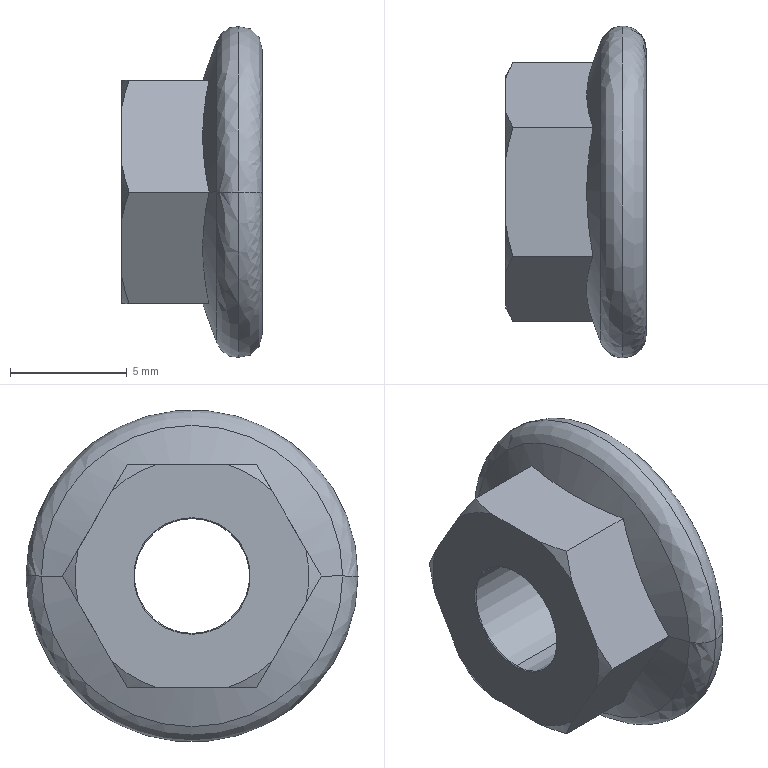Part | SolidWorks | features BaseBody 1 | 1 solid | 26 faces | box 6 x 14.2 x 14.2 mm | volume 511.274 mm3 | cone 12 | plane 8 | spline 4 | cylinder 2 | commonest cylinder face diameters 4.918 x2
STEP:
#1=CARTESIAN_POINT('',(-1.,7.1,0.));
#2=VERTEX_POINT('',#1);
#3=CARTESIAN_POINT('',(-1.,-7.1,0.));
#4=VERTEX_POINT('',#3);
#5=CARTESIAN_POINT('',(-1.,0.,0.));
#6=DIRECTION('',(-1.,0.,0.));
#7=DIRECTION('',(0.,-1.,0.));
#8=AXIS2_PLACEMENT_3D('',#5,#6,#7);
#9=CIRCLE('',#8,7.1);
#10=EDGE_CURVE('',#2,#4,#9,.T.);
#11=ORIENTED_EDGE('',*,*,#10,.F.);
#12=CARTESIAN_POINT('',(0.,6.1,0.));
#13=VERTEX_POINT('',#12);
#14=CARTESIAN_POINT('',(-1.,6.1,0.));
#15=DIRECTION('',(0.,0.,-1.));
#16=DIRECTION('',(0.,1.,0.));
#17=AXIS2_PLACEMENT_3D('',#14,#15,#16);
#18=CIRCLE('',#17,1.);
#19=EDGE_CURVE('',#2,#13,#18,.T.);
#20=ORIENTED_EDGE('',*,*,#19,.T.);
#21=CARTESIAN_POINT('',(0.,-6.1,0.));
#22=VERTEX_POINT('',#21);
#23=CARTESIAN_POINT('',(0.,6.1,0.));
#24=CARTESIAN_POINT('',(0.,6.1,-12.2));
#25=CARTESIAN_POINT('',(0.,-6.1,-12.2));
#26=CARTESIAN_POINT('',(0.,-6.1,0.));
#27=(BOUNDED_CURVE()B_SPLINE_CURVE(3,(#23,#24,#25,#26),.UNSPECIFIED.,.F.,.F.)B_SPLINE_CURVE_WITH_KNOTS((4,4),(0.,1.),.UNSPECIFIED.)CURVE()GEOMETRIC_REPRESENTATION_ITEM()RATIONAL_B_SPLINE_CURVE((1.,0.3333,0.3333,1.))REPRESENTATION_ITEM(''));
#28=EDGE_CURVE('',#13,#22,#27,.T.);
#29=ORIENTED_EDGE('',*,*,#28,.T.);
#30=CARTESIAN_POINT('',(-1.,-6.1,0.));
#31=DIRECTION('',(0.,0.,1.));
#32=DIRECTION('',(0.,-1.,0.));
#33=AXIS2_PLACEMENT_3D('',#30,#31,#32);
#34=CIRCLE('',#33,1.);
#35=EDGE_CURVE('',#4,#22,#34,.T.);
#36=ORIENTED_EDGE('',*,*,#35,.F.);
#37=EDGE_LOOP('',(#11,#20,#29,#36));
#38=FACE_OUTER_BOUND('',#37,.T.);
#39=CARTESIAN_POINT('',(-1.,7.1,0.));
#40=CARTESIAN_POINT('',(-1.,7.1,-14.2));
#41=CARTESIAN_POINT('',(-1.,-7.1,-14.2));
#42=CARTESIAN_POINT('',(-1.,-7.1,0.));
#43=CARTESIAN_POINT('',(-0.4142,7.1,0.));
#44=CARTESIAN_POINT('',(-0.4142,7.1,-14.2));
#45=CARTESIAN_POINT('',(-0.4142,-7.1,-14.2));
#46=CARTESIAN_POINT('',(-0.4142,-7.1,0.));
#47=CARTESIAN_POINT('',(0.,6.686,0.));
#48=CARTESIAN_POINT('',(0.,6.686,-13.372));
#49=CARTESIAN_POINT('',(0.,-6.686,-13.372));
#50=CARTESIAN_POINT('',(0.,-6.686,0.));
#51=CARTESIAN_POINT('',(0.,6.1,0.));
#52=CARTESIAN_POINT('',(0.,6.1,-12.2));
#53=CARTESIAN_POINT('',(0.,-6.1,-12.2));
#54=CARTESIAN_POINT('',(0.,-6.1,0.));
#55=(BOUNDED_SURFACE()B_SPLINE_SURFACE(3,3,((#39,#40,#41,#42),(#43,#44,#45,#46),(#47,#48,#49,#50),(#51,#52,#53,#54)),.UNSPECIFIED.,.F.,.F.,.T.)B_SPLINE_SURFACE_WITH_KNOTS((4,4),(4,4),(0.,1.),(0.,1.),.UNSPECIFIED.)GEOMETRIC_REPRESENTATION_ITEM()RATIONAL_B_SPLINE_SURFACE(((1.,0.3333,0.3333,1.),(0.8047,0.2682,0.2682,0.8047),(0.8047,0.2682,0.2682,0.8047),(1.,0.3333,0.3333,1.)))REPRESENTATION_ITEM('')SURFACE());
#56=ADVANCED_FACE('',(#38),#55,.T.);
#57=CARTESIAN_POINT('',(-1.94,-6.442,0.));
#58=VERTEX_POINT('',#57);
#59=CARTESIAN_POINT('',(-1.94,6.442,0.));
#60=VERTEX_POINT('',#59);
#61=CARTESIAN_POINT('',(-1.94,0.,0.));
#62=DIRECTION('',(1.,0.,0.));
#63=DIRECTION('',(0.,-1.,0.));
#64=AXIS2_PLACEMENT_3D('',#61,#62,#63);
#65=CIRCLE('',#64,6.442);
#66=EDGE_CURVE('',#58,#60,#65,.T.);
#67=ORIENTED_EDGE('',*,*,#66,.T.);
#68=CARTESIAN_POINT('',(-1.,6.1,0.));
#69=DIRECTION('',(0.,0.,-1.));
#70=DIRECTION('',(0.,1.,0.));
#71=AXIS2_PLACEMENT_3D('',#68,#69,#70);
#72=CIRCLE('',#71,1.);
#73=EDGE_CURVE('',#60,#2,#72,.T.);
#74=ORIENTED_EDGE('',*,*,#73,.T.);
#75=ORIENTED_EDGE('',*,*,#10,.T.);
#76=CARTESIAN_POINT('',(-1.,-6.1,0.));
#77=DIRECTION('',(0.,0.,1.));
#78=DIRECTION('',(0.,-1.,0.));
#79=AXIS2_PLACEMENT_3D('',#76,#77,#78);
#80=CIRCLE('',#79,1.);
#81=EDGE_CURVE('',#58,#4,#80,.T.);
#82=ORIENTED_EDGE('',*,*,#81,.F.);
#83=EDGE_LOOP('',(#67,#74,#75,#82));
#84=FACE_OUTER_BOUND('',#83,.T.);
#85=CARTESIAN_POINT('',(-1.94,6.442,0.));
#86=CARTESIAN_POINT('',(-1.94,6.442,-12.884));
#87=CARTESIAN_POINT('',(-1.94,-6.442,-12.884));
#88=CARTESIAN_POINT('',(-1.94,-6.442,0.));
#89=CARTESIAN_POINT('',(-1.791,6.851,0.));
#90=CARTESIAN_POINT('',(-1.791,6.851,-13.701));
#91=CARTESIAN_POINT('',(-1.791,-6.851,-13.701));
#92=CARTESIAN_POINT('',(-1.791,-6.851,0.));
#93=CARTESIAN_POINT('',(-1.435,7.1,0.));
#94=CARTESIAN_POINT('',(-1.435,7.1,-14.2));
#95=CARTESIAN_POINT('',(-1.435,-7.1,-14.2));
#96=CARTESIAN_POINT('',(-1.435,-7.1,0.));
#97=CARTESIAN_POINT('',(-1.,7.1,0.));
#98=CARTESIAN_POINT('',(-1.,7.1,-14.2));
#99=CARTESIAN_POINT('',(-1.,-7.1,-14.2));
#100=CARTESIAN_POINT('',(-1.,-7.1,0.));
#101=(BOUNDED_SURFACE()B_SPLINE_SURFACE(3,3,((#85,#86,#87,#88),(#89,#90,#91,#92),(#93,#94,#95,#96),(#97,#98,#99,#100)),.UNSPECIFIED.,.F.,.F.,.T.)B_SPLINE_SURFACE_WITH_KNOTS((4,4),(4,4),(0.,1.),(0.,1.),.UNSPECIFIED.)GEOMETRIC_REPRESENTATION_ITEM()RATIONAL_B_SPLINE_SURFACE(((1.,0.3333,0.3333,1.),(0.8794,0.2931,0.2931,0.8794),(0.8794,0.2931,0.2931,0.8794),(1.,0.3333,0.3333,1.)))REPRESENTATION_ITEM('')SURFACE());
#102=ADVANCED_FACE('',(#84),#101,.T.);
#103=ORIENTED_EDGE('',*,*,#73,.F.);
#104=CARTESIAN_POINT('',(-1.94,0.,0.));
#105=DIRECTION('',(1.,0.,0.));
#106=DIRECTION('',(0.,-1.,0.));
#107=AXIS2_PLACEMENT_3D('',#104,#105,#106);
#108=CIRCLE('',#107,6.442);
#109=EDGE_CURVE('',#60,#58,#108,.T.);
#110=ORIENTED_EDGE('',*,*,#109,.T.);
#111=ORIENTED_EDGE('',*,*,#81,.T.);
#112=CARTESIAN_POINT('',(-1.,0.,0.));
#113=DIRECTION('',(-1.,0.,0.));
#114=DIRECTION('',(0.,-1.,0.));
#115=AXIS2_PLACEMENT_3D('',#112,#113,#114);
#116=CIRCLE('',#115,7.1);
#117=EDGE_CURVE('',#4,#2,#116,.T.);
#118=ORIENTED_EDGE('',*,*,#117,.T.);
#119=EDGE_LOOP('',(#103,#110,#111,#118));
#120=FACE_OUTER_BOUND('',#119,.T.);
#121=CARTESIAN_POINT('',(-1.94,-6.442,0.));
#122=CARTESIAN_POINT('',(-1.94,-6.442,12.884));
#123=CARTESIAN_POINT('',(-1.94,6.442,12.884));
#124=CARTESIAN_POINT('',(-1.94,6.442,0.));
#125=CARTESIAN_POINT('',(-1.791,-6.851,0.));
#126=CARTESIAN_POINT('',(-1.791,-6.851,13.701));
#127=CARTESIAN_POINT('',(-1.791,6.851,13.701));
#128=CARTESIAN_POINT('',(-1.791,6.851,0.));
#129=CARTESIAN_POINT('',(-1.435,-7.1,0.));
#130=CARTESIAN_POINT('',(-1.435,-7.1,14.2));
#131=CARTESIAN_POINT('',(-1.435,7.1,14.2));
#132=CARTESIAN_POINT('',(-1.435,7.1,0.));
#133=CARTESIAN_POINT('',(-1.,-7.1,0.));
#134=CARTESIAN_POINT('',(-1.,-7.1,14.2));
#135=CARTESIAN_POINT('',(-1.,7.1,14.2));
#136=CARTESIAN_POINT('',(-1.,7.1,0.));
#137=(BOUNDED_SURFACE()B_SPLINE_SURFACE(3,3,((#121,#122,#123,#124),(#125,#126,#127,#128),(#129,#130,#131,#132),(#133,#134,#135,#136)),.UNSPECIFIED.,.F.,.F.,.T.)B_SPLINE_SURFACE_WITH_KNOTS((4,4),(4,4),(0.,1.),(0.,1.),.UNSPECIFIED.)GEOMETRIC_REPRESENTATION_ITEM()RATIONAL_B_SPLINE_SURFACE(((1.,0.3333,0.3333,1.),(0.8794,0.2931,0.2931,0.8794),(0.8794,0.2931,0.2931,0.8794),(1.,0.3333,0.3333,1.)))REPRESENTATION_ITEM('')SURFACE());
#138=ADVANCED_FACE('',(#120),#137,.T.);
#139=CARTESIAN_POINT('',(-0.03571,0.,2.459));
#140=VERTEX_POINT('',#139);
#141=CARTESIAN_POINT('',(-0.03571,0.,-2.459));
#142=VERTEX_POINT('',#141);
#143=CARTESIAN_POINT('',(-0.03571,0.,0.));
#144=DIRECTION('',(1.,0.,0.));
#145=DIRECTION('',(0.,0.,-1.));
#146=AXIS2_PLACEMENT_3D('',#143,#144,#145);
#147=CIRCLE('',#146,2.459);
#148=EDGE_CURVE('',#140,#142,#147,.T.);
#149=ORIENTED_EDGE('',*,*,#148,.F.);
#150=CARTESIAN_POINT('',(0.,0.,2.494));
#151=VERTEX_POINT('',#150);
#152=CARTESIAN_POINT('',(0.,0.,2.494));
#153=DIRECTION('',(0.7071,0.,0.7071));
#154=VECTOR('',#153,1000.);
#155=LINE('',#152,#154);
#156=EDGE_CURVE('',#140,#151,#155,.T.);
#157=ORIENTED_EDGE('',*,*,#156,.T.);
#158=CARTESIAN_POINT('',(0.,0.,-2.494));
#159=VERTEX_POINT('',#158);
#160=CARTESIAN_POINT('',(0.,0.,0.));
#161=DIRECTION('',(1.,0.,0.));
#162=DIRECTION('',(0.,0.,-1.));
#163=AXIS2_PLACEMENT_3D('',#160,#161,#162);
#164=CIRCLE('',#163,2.494);
#165=EDGE_CURVE('',#151,#159,#164,.T.);
#166=ORIENTED_EDGE('',*,*,#165,.T.);
#167=CARTESIAN_POINT('',(0.,0.,-2.494));
#168=DIRECTION('',(0.7071,0.,-0.7071));
#169=VECTOR('',#168,1000.);
#170=LINE('',#167,#169);
#171=EDGE_CURVE('',#142,#159,#170,.T.);
#172=ORIENTED_EDGE('',*,*,#171,.F.);
#173=EDGE_LOOP('',(#149,#157,#166,#172));
#174=FACE_OUTER_BOUND('',#173,.T.);
#175=CARTESIAN_POINT('',(0.,0.,0.));
#176=DIRECTION('',(1.,0.,0.));
#177=DIRECTION('',(0.,0.,-1.));
#178=AXIS2_PLACEMENT_3D('',#175,#176,#177);
#179=CONICAL_SURFACE('',#178,2.494,0.7854);
#180=ADVANCED_FACE('',(#174),#179,.F.);
#181=CARTESIAN_POINT('',(-2.273,-2.763,4.785));
#182=VERTEX_POINT('',#181);
#183=CARTESIAN_POINT('',(-2.273,-5.525,0.));
#184=VERTEX_POINT('',#183);
#185=CARTESIAN_POINT('',(-2.273,-2.763,4.785));
#186=CARTESIAN_POINT('',(-2.441,-3.223,3.987));
#187=CARTESIAN_POINT('',(-2.645,-4.144,2.392));
#188=CARTESIAN_POINT('',(-2.441,-5.065,0.7975));
#189=CARTESIAN_POINT('',(-2.273,-5.525,0.));
#190=B_SPLINE_CURVE_WITH_KNOTS('',3,(#185,#186,#187,#188,#189),.UNSPECIFIED.,.F.,.F.,(4,1,4),(0.,0.002762,0.005525),.UNSPECIFIED.);
#191=EDGE_CURVE('',#182,#184,#190,.T.);
#192=ORIENTED_EDGE('',*,*,#191,.T.);
#193=CARTESIAN_POINT('',(-1.94,-6.442,0.));
#194=DIRECTION('',(0.342,-0.9397,0.));
#195=VECTOR('',#194,1000.);
#196=LINE('',#193,#195);
#197=EDGE_CURVE('',#184,#58,#196,.T.);
#198=ORIENTED_EDGE('',*,*,#197,.T.);
#199=ORIENTED_EDGE('',*,*,#109,.F.);
#200=CARTESIAN_POINT('',(-2.273,5.525,0.));
#201=VERTEX_POINT('',#200);
#202=CARTESIAN_POINT('',(-1.94,6.442,0.));
#203=DIRECTION('',(0.342,0.9397,0.));
#204=VECTOR('',#203,1000.);
#205=LINE('',#202,#204);
#206=EDGE_CURVE('',#201,#60,#205,.T.);
#207=ORIENTED_EDGE('',*,*,#206,.F.);
#208=CARTESIAN_POINT('',(-2.273,2.763,4.785));
#209=VERTEX_POINT('',#208);
#210=CARTESIAN_POINT('',(-2.273,5.525,0.));
#211=CARTESIAN_POINT('',(-2.441,5.065,0.7975));
#212=CARTESIAN_POINT('',(-2.645,4.144,2.392));
#213=CARTESIAN_POINT('',(-2.441,3.223,3.987));
#214=CARTESIAN_POINT('',(-2.273,2.763,4.785));
#215=B_SPLINE_CURVE_WITH_KNOTS('',3,(#210,#211,#212,#213,#214),.UNSPECIFIED.,.F.,.F.,(4,1,4),(0.,0.002762,0.005525),.UNSPECIFIED.);
#216=EDGE_CURVE('',#201,#209,#215,.T.);
#217=ORIENTED_EDGE('',*,*,#216,.T.);
#218=CARTESIAN_POINT('',(-2.273,2.763,4.785));
#219=CARTESIAN_POINT('',(-2.441,1.842,4.785));
#220=CARTESIAN_POINT('',(-2.645,0.000000035,4.785));
#221=CARTESIAN_POINT('',(-2.441,-1.842,4.785));
#222=CARTESIAN_POINT('',(-2.273,-2.763,4.785));
#223=B_SPLINE_CURVE_WITH_KNOTS('',3,(#218,#219,#220,#221,#222),.UNSPECIFIED.,.F.,.F.,(4,1,4),(0.,0.002763,0.005525),.UNSPECIFIED.);
#224=EDGE_CURVE('',#209,#182,#223,.T.);
#225=ORIENTED_EDGE('',*,*,#224,.T.);
#226=EDGE_LOOP('',(#192,#198,#199,#207,#217,#225));
#227=FACE_OUTER_BOUND('',#226,.T.);
#228=CARTESIAN_POINT('',(-1.94,0.,0.));
#229=DIRECTION('',(1.,0.,0.));
#230=DIRECTION('',(0.,1.,0.));
#231=AXIS2_PLACEMENT_3D('',#228,#229,#230);
#232=CONICAL_SURFACE('',#231,6.442,1.222);
#233=ADVANCED_FACE('',(#227),#232,.T.);
#234=ORIENTED_EDGE('',*,*,#148,.T.);
#235=CARTESIAN_POINT('',(-5.964,0.,-2.459));
#236=VERTEX_POINT('',#235);
#237=CARTESIAN_POINT('',(0.,0.,-2.459));
#238=DIRECTION('',(-1.,0.,0.));
#239=VECTOR('',#238,1000.);
#240=LINE('',#237,#239);
#241=EDGE_CURVE('',#142,#236,#240,.T.);
#242=ORIENTED_EDGE('',*,*,#241,.T.);
#243=CARTESIAN_POINT('',(-5.964,0.,2.459));
#244=VERTEX_POINT('',#243);
#245=CARTESIAN_POINT('',(-5.964,0.,0.));
#246=DIRECTION('',(1.,0.,0.));
#247=DIRECTION('',(0.,0.,1.));
#248=AXIS2_PLACEMENT_3D('',#245,#246,#247);
#249=CIRCLE('',#248,2.459);
#250=EDGE_CURVE('',#244,#236,#249,.T.);
#251=ORIENTED_EDGE('',*,*,#250,.F.);
#252=CARTESIAN_POINT('',(0.,0.,2.459));
#253=DIRECTION('',(-1.,0.,0.));
#254=VECTOR('',#253,1000.);
#255=LINE('',#252,#254);
#256=EDGE_CURVE('',#140,#244,#255,.T.);
#257=ORIENTED_EDGE('',*,*,#256,.F.);
#258=EDGE_LOOP('',(#234,#242,#251,#257));
#259=FACE_OUTER_BOUND('',#258,.T.);
#260=CARTESIAN_POINT('',(0.,0.,0.));
#261=DIRECTION('',(-1.,0.,0.));
#262=DIRECTION('',(0.,0.,1.));
#263=AXIS2_PLACEMENT_3D('',#260,#261,#262);
#264=CYLINDRICAL_SURFACE('',#263,2.459);
#265=ADVANCED_FACE('',(#259),#264,.F.);
#266=ORIENTED_EDGE('',*,*,#250,.T.);
#267=CARTESIAN_POINT('',(-6.,0.,-2.494));
#268=VERTEX_POINT('',#267);
#269=CARTESIAN_POINT('',(-6.,0.,-2.494));
#270=DIRECTION('',(-0.7071,0.,-0.7071));
#271=VECTOR('',#270,1000.);
#272=LINE('',#269,#271);
#273=EDGE_CURVE('',#236,#268,#272,.T.);
#274=ORIENTED_EDGE('',*,*,#273,.T.);
#275=CARTESIAN_POINT('',(-6.,0.,2.494));
#276=VERTEX_POINT('',#275);
#277=CARTESIAN_POINT('',(-6.,0.,0.));
#278=DIRECTION('',(1.,0.,0.));
#279=DIRECTION('',(0.,0.,1.));
#280=AXIS2_PLACEMENT_3D('',#277,#278,#279);
#281=CIRCLE('',#280,2.494);
#282=EDGE_CURVE('',#276,#268,#281,.T.);
#283=ORIENTED_EDGE('',*,*,#282,.F.);
#284=CARTESIAN_POINT('',(-6.,0.,2.494));
#285=DIRECTION('',(-0.7071,0.,0.7071));
#286=VECTOR('',#285,1000.);
#287=LINE('',#284,#286);
#288=EDGE_CURVE('',#244,#276,#287,.T.);
#289=ORIENTED_EDGE('',*,*,#288,.F.);
#290=EDGE_LOOP('',(#266,#274,#283,#289));
#291=FACE_OUTER_BOUND('',#290,.T.);
#292=CARTESIAN_POINT('',(-6.,0.,0.));
#293=DIRECTION('',(-1.,0.,0.));
#294=DIRECTION('',(0.,0.,1.));
#295=AXIS2_PLACEMENT_3D('',#292,#293,#294);
#296=CONICAL_SURFACE('',#295,2.494,0.7854);
#297=ADVANCED_FACE('',(#291),#296,.F.);
#298=ORIENTED_EDGE('',*,*,#28,.F.);
#299=CARTESIAN_POINT('',(0.,-6.1,0.));
#300=CARTESIAN_POINT('',(0.,-6.1,12.2));
#301=CARTESIAN_POINT('',(0.,6.1,12.2));
#302=CARTESIAN_POINT('',(0.,6.1,0.));
#303=(BOUNDED_CURVE()B_SPLINE_CURVE(3,(#299,#300,#301,#302),.UNSPECIFIED.,.F.,.F.)B_SPLINE_CURVE_WITH_KNOTS((4,4),(0.,1.),.UNSPECIFIED.)CURVE()GEOMETRIC_REPRESENTATION_ITEM()RATIONAL_B_SPLINE_CURVE((1.,0.3333,0.3333,1.))REPRESENTATION_ITEM(''));
#304=EDGE_CURVE('',#22,#13,#303,.T.);
#305=ORIENTED_EDGE('',*,*,#304,.F.);
#306=EDGE_LOOP('',(#298,#305));
#307=FACE_OUTER_BOUND('',#306,.T.);
#308=CARTESIAN_POINT('',(0.,0.,0.));
#309=DIRECTION('',(1.,0.,0.));
#310=DIRECTION('',(0.,0.,-1.));
#311=AXIS2_PLACEMENT_3D('',#308,#309,#310);
#312=CIRCLE('',#311,2.494);
#313=EDGE_CURVE('',#159,#151,#312,.T.);
#314=ORIENTED_EDGE('',*,*,#313,.F.);
#315=ORIENTED_EDGE('',*,*,#165,.F.);
#316=EDGE_LOOP('',(#314,#315));
#317=FACE_BOUND('',#316,.T.);
#318=CARTESIAN_POINT('',(0.,0.,0.));
#319=DIRECTION('',(-1.,0.,0.));
#320=DIRECTION('',(0.,-1.,0.));
#321=AXIS2_PLACEMENT_3D('',#318,#319,#320);
#322=PLANE('',#321);
#323=ADVANCED_FACE('',(#307,#317),#322,.F.);
#324=ORIENTED_EDGE('',*,*,#19,.F.);
#325=ORIENTED_EDGE('',*,*,#117,.F.);
#326=ORIENTED_EDGE('',*,*,#35,.T.);
#327=ORIENTED_EDGE('',*,*,#304,.T.);
#328=EDGE_LOOP('',(#324,#325,#326,#327));
#329=FACE_OUTER_BOUND('',#328,.T.);
#330=CARTESIAN_POINT('',(-1.,-7.1,0.));
#331=CARTESIAN_POINT('',(-1.,-7.1,14.2));
#332=CARTESIAN_POINT('',(-1.,7.1,14.2));
#333=CARTESIAN_POINT('',(-1.,7.1,0.));
#334=CARTESIAN_POINT('',(-0.4142,-7.1,0.));
#335=CARTESIAN_POINT('',(-0.4142,-7.1,14.2));
#336=CARTESIAN_POINT('',(-0.4142,7.1,14.2));
#337=CARTESIAN_POINT('',(-0.4142,7.1,0.));
#338=CARTESIAN_POINT('',(0.,-6.686,0.));
#339=CARTESIAN_POINT('',(0.,-6.686,13.372));
#340=CARTESIAN_POINT('',(0.,6.686,13.372));
#341=CARTESIAN_POINT('',(0.,6.686,0.));
#342=CARTESIAN_POINT('',(0.,-6.1,0.));
#343=CARTESIAN_POINT('',(0.,-6.1,12.2));
#344=CARTESIAN_POINT('',(0.,6.1,12.2));
#345=CARTESIAN_POINT('',(0.,6.1,0.));
#346=(BOUNDED_SURFACE()B_SPLINE_SURFACE(3,3,((#330,#331,#332,#333),(#334,#335,#336,#337),(#338,#339,#340,#341),(#342,#343,#344,#345)),.UNSPECIFIED.,.F.,.F.,.T.)B_SPLINE_SURFACE_WITH_KNOTS((4,4),(4,4),(0.,1.),(0.,1.),.UNSPECIFIED.)GEOMETRIC_REPRESENTATION_ITEM()RATIONAL_B_SPLINE_SURFACE(((1.,0.3333,0.3333,1.),(0.8047,0.2682,0.2682,0.8047),(0.8047,0.2682,0.2682,0.8047),(1.,0.3333,0.3333,1.)))REPRESENTATION_ITEM('')SURFACE());
#347=ADVANCED_FACE('',(#329),#346,.T.);
#348=ORIENTED_EDGE('',*,*,#156,.F.);
#349=CARTESIAN_POINT('',(-0.03571,0.,0.));
#350=DIRECTION('',(1.,0.,0.));
#351=DIRECTION('',(0.,0.,-1.));
#352=AXIS2_PLACEMENT_3D('',#349,#350,#351);
#353=CIRCLE('',#352,2.459);
#354=EDGE_CURVE('',#142,#140,#353,.T.);
#355=ORIENTED_EDGE('',*,*,#354,.F.);
#356=ORIENTED_EDGE('',*,*,#171,.T.);
#357=ORIENTED_EDGE('',*,*,#313,.T.);
#358=EDGE_LOOP('',(#348,#355,#356,#357));
#359=FACE_OUTER_BOUND('',#358,.T.);
#360=CARTESIAN_POINT('',(0.,0.,0.));
#361=DIRECTION('',(1.,0.,0.));
#362=DIRECTION('',(0.,0.,-1.));
#363=AXIS2_PLACEMENT_3D('',#360,#361,#362);
#364=CONICAL_SURFACE('',#363,2.494,0.7854);
#365=ADVANCED_FACE('',(#359),#364,.F.);
#366=ORIENTED_EDGE('',*,*,#197,.F.);
#367=CARTESIAN_POINT('',(-2.273,-2.763,-4.785));
#368=VERTEX_POINT('',#367);
#369=CARTESIAN_POINT('',(-2.273,-5.525,0.));
#370=CARTESIAN_POINT('',(-2.441,-5.065,-0.7975));
#371=CARTESIAN_POINT('',(-2.645,-4.144,-2.392));
#372=CARTESIAN_POINT('',(-2.441,-3.223,-3.987));
#373=CARTESIAN_POINT('',(-2.273,-2.763,-4.785));
#374=B_SPLINE_CURVE_WITH_KNOTS('',3,(#369,#370,#371,#372,#373),.UNSPECIFIED.,.F.,.F.,(4,1,4),(0.,0.002762,0.005525),.UNSPECIFIED.);
#375=EDGE_CURVE('',#184,#368,#374,.T.);
#376=ORIENTED_EDGE('',*,*,#375,.T.);
#377=CARTESIAN_POINT('',(-2.273,2.762,-4.785));
#378=VERTEX_POINT('',#377);
#379=CARTESIAN_POINT('',(-2.273,-2.763,-4.785));
#380=CARTESIAN_POINT('',(-2.441,-1.842,-4.785));
#381=CARTESIAN_POINT('',(-2.645,-0.000000071,-4.785));
#382=CARTESIAN_POINT('',(-2.441,1.842,-4.785));
#383=CARTESIAN_POINT('',(-2.273,2.762,-4.785));
#384=B_SPLINE_CURVE_WITH_KNOTS('',3,(#379,#380,#381,#382,#383),.UNSPECIFIED.,.F.,.F.,(4,1,4),(0.,0.002763,0.005525),.UNSPECIFIED.);
#385=EDGE_CURVE('',#368,#378,#384,.T.);
#386=ORIENTED_EDGE('',*,*,#385,.T.);
#387=CARTESIAN_POINT('',(-2.273,2.762,-4.785));
#388=CARTESIAN_POINT('',(-2.441,3.223,-3.987));
#389=CARTESIAN_POINT('',(-2.645,4.144,-2.392));
#390=CARTESIAN_POINT('',(-2.441,5.065,-0.7975));
#391=CARTESIAN_POINT('',(-2.273,5.525,0.));
#392=B_SPLINE_CURVE_WITH_KNOTS('',3,(#387,#388,#389,#390,#391),.UNSPECIFIED.,.F.,.F.,(4,1,4),(0.,0.002763,0.005525),.UNSPECIFIED.);
#393=EDGE_CURVE('',#378,#201,#392,.T.);
#394=ORIENTED_EDGE('',*,*,#393,.T.);
#395=ORIENTED_EDGE('',*,*,#206,.T.);
#396=ORIENTED_EDGE('',*,*,#66,.F.);
#397=EDGE_LOOP('',(#366,#376,#386,#394,#395,#396));
#398=FACE_OUTER_BOUND('',#397,.T.);
#399=CARTESIAN_POINT('',(-1.94,0.,0.));
#400=DIRECTION('',(1.,0.,0.));
#401=DIRECTION('',(0.,1.,0.));
#402=AXIS2_PLACEMENT_3D('',#399,#400,#401);
#403=CONICAL_SURFACE('',#402,6.442,1.222);
#404=ADVANCED_FACE('',(#398),#403,.T.);
#405=ORIENTED_EDGE('',*,*,#241,.F.);
#406=ORIENTED_EDGE('',*,*,#354,.T.);
#407=ORIENTED_EDGE('',*,*,#256,.T.);
#408=CARTESIAN_POINT('',(-5.964,0.,0.));
#409=DIRECTION('',(1.,0.,0.));
#410=DIRECTION('',(0.,0.,1.));
#411=AXIS2_PLACEMENT_3D('',#408,#409,#410);
#412=CIRCLE('',#411,2.459);
#413=EDGE_CURVE('',#236,#244,#412,.T.);
#414=ORIENTED_EDGE('',*,*,#413,.F.);
#415=EDGE_LOOP('',(#405,#406,#407,#414));
#416=FACE_OUTER_BOUND('',#415,.T.);
#417=CARTESIAN_POINT('',(0.,0.,0.));
#418=DIRECTION('',(-1.,0.,0.));
#419=DIRECTION('',(0.,0.,1.));
#420=AXIS2_PLACEMENT_3D('',#417,#418,#419);
#421=CYLINDRICAL_SURFACE('',#420,2.459);
#422=ADVANCED_FACE('',(#416),#421,.F.);
#423=CARTESIAN_POINT('',(-5.697,-2.763,4.785));
#424=VERTEX_POINT('',#423);
#425=CARTESIAN_POINT('',(-6.,-2.763,4.785));
#426=DIRECTION('',(-1.,0.,0.));
#427=VECTOR('',#426,1000.);
#428=LINE('',#425,#427);
#429=EDGE_CURVE('',#182,#424,#428,.T.);
#430=ORIENTED_EDGE('',*,*,#429,.F.);
#431=ORIENTED_EDGE('',*,*,#224,.F.);
#432=CARTESIAN_POINT('',(-5.697,2.763,4.785));
#433=VERTEX_POINT('',#432);
#434=CARTESIAN_POINT('',(-6.,2.763,4.785));
#435=DIRECTION('',(1.,0.,0.));
#436=VECTOR('',#435,1000.);
#437=LINE('',#434,#436);
#438=EDGE_CURVE('',#433,#209,#437,.T.);
#439=ORIENTED_EDGE('',*,*,#438,.F.);
#440=CARTESIAN_POINT('',(-6.,1.451,4.785));
#441=VERTEX_POINT('',#440);
#442=CARTESIAN_POINT('',(-6.,1.451,4.785));
#443=CARTESIAN_POINT('',(-5.926,1.894,4.785));
#444=CARTESIAN_POINT('',(-5.822,2.331,4.785));
#445=CARTESIAN_POINT('',(-5.697,2.763,4.785));
#446=B_SPLINE_CURVE_WITH_KNOTS('',3,(#442,#443,#444,#445),.UNSPECIFIED.,.F.,.F.,(4,4),(0.,0.001346),.UNSPECIFIED.);
#447=EDGE_CURVE('',#441,#433,#446,.T.);
#448=ORIENTED_EDGE('',*,*,#447,.F.);
#449=CARTESIAN_POINT('',(-6.,-1.451,4.785));
#450=VERTEX_POINT('',#449);
#451=CARTESIAN_POINT('',(-6.,-2.762,4.785));
#452=DIRECTION('',(0.,1.,0.));
#453=VECTOR('',#452,1000.);
#454=LINE('',#451,#453);
#455=EDGE_CURVE('',#450,#441,#454,.T.);
#456=ORIENTED_EDGE('',*,*,#455,.F.);
#457=CARTESIAN_POINT('',(-5.697,-2.763,4.785));
#458=CARTESIAN_POINT('',(-5.822,-2.331,4.785));
#459=CARTESIAN_POINT('',(-5.926,-1.894,4.785));
#460=CARTESIAN_POINT('',(-6.,-1.451,4.785));
#461=B_SPLINE_CURVE_WITH_KNOTS('',3,(#457,#458,#459,#460),.UNSPECIFIED.,.F.,.F.,(4,4),(0.,0.001346),.UNSPECIFIED.);
#462=EDGE_CURVE('',#424,#450,#461,.T.);
#463=ORIENTED_EDGE('',*,*,#462,.F.);
#464=EDGE_LOOP('',(#430,#431,#439,#448,#456,#463));
#465=FACE_OUTER_BOUND('',#464,.T.);
#466=CARTESIAN_POINT('',(-6.,-2.762,4.785));
#467=DIRECTION('',(0.,0.,-1.));
#468=DIRECTION('',(0.,1.,0.));
#469=AXIS2_PLACEMENT_3D('',#466,#467,#468);
#470=PLANE('',#469);
#471=ADVANCED_FACE('',(#465),#470,.F.);
#472=ORIENTED_EDGE('',*,*,#438,.T.);
#473=ORIENTED_EDGE('',*,*,#216,.F.);
#474=CARTESIAN_POINT('',(-5.697,5.525,0.000000043));
#475=VERTEX_POINT('',#474);
#476=CARTESIAN_POINT('',(-6.,5.525,0.));
#477=DIRECTION('',(1.,0.,0.));
#478=VECTOR('',#477,1000.);
#479=LINE('',#476,#478);
#480=EDGE_CURVE('',#475,#201,#479,.T.);
#481=ORIENTED_EDGE('',*,*,#480,.F.);
#482=CARTESIAN_POINT('',(-6.,4.869,1.136));
#483=VERTEX_POINT('',#482);
#484=CARTESIAN_POINT('',(-6.,4.869,1.136));
#485=CARTESIAN_POINT('',(-5.926,5.091,0.7518));
#486=CARTESIAN_POINT('',(-5.822,5.309,0.3738));
#487=CARTESIAN_POINT('',(-5.697,5.525,0.000000043));
#488=B_SPLINE_CURVE_WITH_KNOTS('',3,(#484,#485,#486,#487),.UNSPECIFIED.,.F.,.F.,(4,4),(0.,0.001346),.UNSPECIFIED.);
#489=EDGE_CURVE('',#483,#475,#488,.T.);
#490=ORIENTED_EDGE('',*,*,#489,.F.);
#491=CARTESIAN_POINT('',(-6.,3.418,3.649));
#492=VERTEX_POINT('',#491);
#493=CARTESIAN_POINT('',(-6.,2.763,4.785));
#494=DIRECTION('',(0.,0.5,-0.866));
#495=VECTOR('',#494,1000.);
#496=LINE('',#493,#495);
#497=EDGE_CURVE('',#492,#483,#496,.T.);
#498=ORIENTED_EDGE('',*,*,#497,.F.);
#499=CARTESIAN_POINT('',(-5.697,2.763,4.785));
#500=CARTESIAN_POINT('',(-5.822,2.978,4.411));
#501=CARTESIAN_POINT('',(-5.926,3.197,4.033));
#502=CARTESIAN_POINT('',(-6.,3.418,3.649));
#503=B_SPLINE_CURVE_WITH_KNOTS('',3,(#499,#500,#501,#502),.UNSPECIFIED.,.F.,.F.,(4,4),(0.,0.001346),.UNSPECIFIED.);
#504=EDGE_CURVE('',#433,#492,#503,.T.);
#505=ORIENTED_EDGE('',*,*,#504,.F.);
#506=EDGE_LOOP('',(#472,#473,#481,#490,#498,#505));
#507=FACE_OUTER_BOUND('',#506,.T.);
#508=CARTESIAN_POINT('',(-6.,2.763,4.785));
#509=DIRECTION('',(0.,-0.866,-0.5));
#510=DIRECTION('',(0.,0.5,-0.866));
#511=AXIS2_PLACEMENT_3D('',#508,#509,#510);
#512=PLANE('',#511);
#513=ADVANCED_FACE('',(#507),#512,.F.);
#514=CARTESIAN_POINT('',(-5.697,-5.525,-0.000000043));
#515=VERTEX_POINT('',#514);
#516=CARTESIAN_POINT('',(-6.,-5.525,0.));
#517=DIRECTION('',(-1.,0.,0.));
#518=VECTOR('',#517,1000.);
#519=LINE('',#516,#518);
#520=EDGE_CURVE('',#184,#515,#519,.T.);
#521=ORIENTED_EDGE('',*,*,#520,.F.);
#522=ORIENTED_EDGE('',*,*,#191,.F.);
#523=ORIENTED_EDGE('',*,*,#429,.T.);
#524=CARTESIAN_POINT('',(-6.,-3.418,3.649));
#525=VERTEX_POINT('',#524);
#526=CARTESIAN_POINT('',(-6.,-3.418,3.649));
#527=CARTESIAN_POINT('',(-5.926,-3.197,4.033));
#528=CARTESIAN_POINT('',(-5.822,-2.978,4.411));
#529=CARTESIAN_POINT('',(-5.697,-2.763,4.785));
#530=B_SPLINE_CURVE_WITH_KNOTS('',3,(#526,#527,#528,#529),.UNSPECIFIED.,.F.,.F.,(4,4),(0.,0.001346),.UNSPECIFIED.);
#531=EDGE_CURVE('',#525,#424,#530,.T.);
#532=ORIENTED_EDGE('',*,*,#531,.F.);
#533=CARTESIAN_POINT('',(-6.,-4.869,1.136));
#534=VERTEX_POINT('',#533);
#535=CARTESIAN_POINT('',(-6.,-5.525,0.));
#536=DIRECTION('',(0.,0.5,0.866));
#537=VECTOR('',#536,1000.);
#538=LINE('',#535,#537);
#539=EDGE_CURVE('',#534,#525,#538,.T.);
#540=ORIENTED_EDGE('',*,*,#539,.F.);
#541=CARTESIAN_POINT('',(-5.697,-5.525,-0.000000043));
#542=CARTESIAN_POINT('',(-5.822,-5.309,0.3738));
#543=CARTESIAN_POINT('',(-5.926,-5.091,0.7518));
#544=CARTESIAN_POINT('',(-6.,-4.869,1.136));
#545=B_SPLINE_CURVE_WITH_KNOTS('',3,(#541,#542,#543,#544),.UNSPECIFIED.,.F.,.F.,(4,4),(0.,0.001346),.UNSPECIFIED.);
#546=EDGE_CURVE('',#515,#534,#545,.T.);
#547=ORIENTED_EDGE('',*,*,#546,.F.);
#548=EDGE_LOOP('',(#521,#522,#523,#532,#540,#547));
#549=FACE_OUTER_BOUND('',#548,.T.);
#550=CARTESIAN_POINT('',(-6.,-5.525,0.));
#551=DIRECTION('',(0.,0.866,-0.5));
#552=DIRECTION('',(0.,0.5,0.866));
#553=AXIS2_PLACEMENT_3D('',#550,#551,#552);
#554=PLANE('',#553);
#555=ADVANCED_FACE('',(#549),#554,.F.);
#556=ORIENTED_EDGE('',*,*,#480,.T.);
#557=ORIENTED_EDGE('',*,*,#393,.F.);
#558=CARTESIAN_POINT('',(-5.697,2.763,-4.785));
#559=VERTEX_POINT('',#558);
#560=CARTESIAN_POINT('',(-6.,2.762,-4.785));
#561=DIRECTION('',(1.,0.,0.));
#562=VECTOR('',#561,1000.);
#563=LINE('',#560,#562);
#564=EDGE_CURVE('',#559,#378,#563,.T.);
#565=ORIENTED_EDGE('',*,*,#564,.F.);
#566=CARTESIAN_POINT('',(-6.,3.418,-3.649));
#567=VERTEX_POINT('',#566);
#568=CARTESIAN_POINT('',(-6.,3.418,-3.649));
#569=CARTESIAN_POINT('',(-5.926,3.197,-4.033));
#570=CARTESIAN_POINT('',(-5.822,2.978,-4.411));
#571=CARTESIAN_POINT('',(-5.697,2.763,-4.785));
#572=B_SPLINE_CURVE_WITH_KNOTS('',3,(#568,#569,#570,#571),.UNSPECIFIED.,.F.,.F.,(4,4),(0.,0.001346),.UNSPECIFIED.);
#573=EDGE_CURVE('',#567,#559,#572,.T.);
#574=ORIENTED_EDGE('',*,*,#573,.F.);
#575=CARTESIAN_POINT('',(-6.,4.869,-1.136));
#576=VERTEX_POINT('',#575);
#577=CARTESIAN_POINT('',(-6.,5.525,0.));
#578=DIRECTION('',(0.,-0.5,-0.866));
#579=VECTOR('',#578,1000.);
#580=LINE('',#577,#579);
#581=EDGE_CURVE('',#576,#567,#580,.T.);
#582=ORIENTED_EDGE('',*,*,#581,.F.);
#583=CARTESIAN_POINT('',(-5.697,5.525,0.000000043));
#584=CARTESIAN_POINT('',(-5.822,5.309,-0.3738));
#585=CARTESIAN_POINT('',(-5.926,5.091,-0.7518));
#586=CARTESIAN_POINT('',(-6.,4.869,-1.136));
#587=B_SPLINE_CURVE_WITH_KNOTS('',3,(#583,#584,#585,#586),.UNSPECIFIED.,.F.,.F.,(4,4),(0.,0.001346),.UNSPECIFIED.);
#588=EDGE_CURVE('',#475,#576,#587,.T.);
#589=ORIENTED_EDGE('',*,*,#588,.F.);
#590=EDGE_LOOP('',(#556,#557,#565,#574,#582,#589));
#591=FACE_OUTER_BOUND('',#590,.T.);
#592=CARTESIAN_POINT('',(-6.,5.525,0.));
#593=DIRECTION('',(0.,-0.866,0.5));
#594=DIRECTION('',(0.,-0.5,-0.866));
#595=AXIS2_PLACEMENT_3D('',#592,#593,#594);
#596=PLANE('',#595);
#597=ADVANCED_FACE('',(#591),#596,.F.);
#598=ORIENTED_EDGE('',*,*,#564,.T.);
#599=ORIENTED_EDGE('',*,*,#385,.F.);
#600=CARTESIAN_POINT('',(-5.697,-2.762,-4.785));
#601=VERTEX_POINT('',#600);
#602=CARTESIAN_POINT('',(-6.,-2.762,-4.785));
#603=DIRECTION('',(1.,0.,0.));
#604=VECTOR('',#603,1000.);
#605=LINE('',#602,#604);
#606=EDGE_CURVE('',#601,#368,#605,.T.);
#607=ORIENTED_EDGE('',*,*,#606,.F.);
#608=CARTESIAN_POINT('',(-6.,-1.451,-4.785));
#609=VERTEX_POINT('',#608);
#610=CARTESIAN_POINT('',(-6.,-1.451,-4.785));
#611=CARTESIAN_POINT('',(-5.926,-1.894,-4.785));
#612=CARTESIAN_POINT('',(-5.822,-2.331,-4.785));
#613=CARTESIAN_POINT('',(-5.697,-2.762,-4.785));
#614=B_SPLINE_CURVE_WITH_KNOTS('',3,(#610,#611,#612,#613),.UNSPECIFIED.,.F.,.F.,(4,4),(0.,0.001346),.UNSPECIFIED.);
#615=EDGE_CURVE('',#609,#601,#614,.T.);
#616=ORIENTED_EDGE('',*,*,#615,.F.);
#617=CARTESIAN_POINT('',(-6.,1.451,-4.785));
#618=VERTEX_POINT('',#617);
#619=CARTESIAN_POINT('',(-6.,2.763,-4.785));
#620=DIRECTION('',(0.,-1.,0.));
#621=VECTOR('',#620,1000.);
#622=LINE('',#619,#621);
#623=EDGE_CURVE('',#618,#609,#622,.T.);
#624=ORIENTED_EDGE('',*,*,#623,.F.);
#625=CARTESIAN_POINT('',(-5.697,2.763,-4.785));
#626=CARTESIAN_POINT('',(-5.822,2.331,-4.785));
#627=CARTESIAN_POINT('',(-5.926,1.894,-4.785));
#628=CARTESIAN_POINT('',(-6.,1.451,-4.785));
#629=B_SPLINE_CURVE_WITH_KNOTS('',3,(#625,#626,#627,#628),.UNSPECIFIED.,.F.,.F.,(4,4),(0.,0.001346),.UNSPECIFIED.);
#630=EDGE_CURVE('',#559,#618,#629,.T.);
#631=ORIENTED_EDGE('',*,*,#630,.F.);
#632=EDGE_LOOP('',(#598,#599,#607,#616,#624,#631));
#633=FACE_OUTER_BOUND('',#632,.T.);
#634=CARTESIAN_POINT('',(-6.,2.763,-4.785));
#635=DIRECTION('',(0.,0.,1.));
#636=DIRECTION('',(0.,-1.,0.));
#637=AXIS2_PLACEMENT_3D('',#634,#635,#636);
#638=PLANE('',#637);
#639=ADVANCED_FACE('',(#633),#638,.F.);
#640=ORIENTED_EDGE('',*,*,#606,.T.);
#641=ORIENTED_EDGE('',*,*,#375,.F.);
#642=ORIENTED_EDGE('',*,*,#520,.T.);
#643=CARTESIAN_POINT('',(-6.,-4.869,-1.136));
#644=VERTEX_POINT('',#643);
#645=CARTESIAN_POINT('',(-6.,-4.869,-1.136));
#646=CARTESIAN_POINT('',(-5.926,-5.091,-0.7518));
#647=CARTESIAN_POINT('',(-5.822,-5.309,-0.3738));
#648=CARTESIAN_POINT('',(-5.697,-5.525,-0.000000043));
#649=B_SPLINE_CURVE_WITH_KNOTS('',3,(#645,#646,#647,#648),.UNSPECIFIED.,.F.,.F.,(4,4),(0.,0.001346),.UNSPECIFIED.);
#650=EDGE_CURVE('',#644,#515,#649,.T.);
#651=ORIENTED_EDGE('',*,*,#650,.F.);
#652=CARTESIAN_POINT('',(-6.,-3.418,-3.649));
#653=VERTEX_POINT('',#652);
#654=CARTESIAN_POINT('',(-6.,-2.762,-4.785));
#655=DIRECTION('',(0.,-0.5,0.866));
#656=VECTOR('',#655,1000.);
#657=LINE('',#654,#656);
#658=EDGE_CURVE('',#653,#644,#657,.T.);
#659=ORIENTED_EDGE('',*,*,#658,.F.);
#660=CARTESIAN_POINT('',(-5.697,-2.762,-4.785));
#661=CARTESIAN_POINT('',(-5.822,-2.978,-4.411));
#662=CARTESIAN_POINT('',(-5.926,-3.197,-4.033));
#663=CARTESIAN_POINT('',(-6.,-3.418,-3.649));
#664=B_SPLINE_CURVE_WITH_KNOTS('',3,(#660,#661,#662,#663),.UNSPECIFIED.,.F.,.F.,(4,4),(0.,0.001346),.UNSPECIFIED.);
#665=EDGE_CURVE('',#601,#653,#664,.T.);
#666=ORIENTED_EDGE('',*,*,#665,.F.);
#667=EDGE_LOOP('',(#640,#641,#642,#651,#659,#666));
#668=FACE_OUTER_BOUND('',#667,.T.);
#669=CARTESIAN_POINT('',(-6.,-2.762,-4.785));
#670=DIRECTION('',(0.,0.866,0.5));
#671=DIRECTION('',(0.,-0.5,0.866));
#672=AXIS2_PLACEMENT_3D('',#669,#670,#671);
#673=PLANE('',#672);
#674=ADVANCED_FACE('',(#668),#673,.F.);
#675=ORIENTED_EDGE('',*,*,#273,.F.);
#676=ORIENTED_EDGE('',*,*,#413,.T.);
#677=ORIENTED_EDGE('',*,*,#288,.T.);
#678=CARTESIAN_POINT('',(-6.,0.,0.));
#679=DIRECTION('',(1.,0.,0.));
#680=DIRECTION('',(0.,0.,1.));
#681=AXIS2_PLACEMENT_3D('',#678,#679,#680);
#682=CIRCLE('',#681,2.494);
#683=EDGE_CURVE('',#268,#276,#682,.T.);
#684=ORIENTED_EDGE('',*,*,#683,.F.);
#685=EDGE_LOOP('',(#675,#676,#677,#684));
#686=FACE_OUTER_BOUND('',#685,.T.);
#687=CARTESIAN_POINT('',(-6.,0.,0.));
#688=DIRECTION('',(-1.,0.,0.));
#689=DIRECTION('',(0.,0.,1.));
#690=AXIS2_PLACEMENT_3D('',#687,#688,#689);
#691=CONICAL_SURFACE('',#690,2.494,0.7854);
#692=ADVANCED_FACE('',(#686),#691,.F.);
#693=ORIENTED_EDGE('',*,*,#539,.T.);
#694=CARTESIAN_POINT('',(-6.,0.,0.));
#695=DIRECTION('',(-1.,0.,0.));
#696=DIRECTION('',(0.,0.,-1.));
#697=AXIS2_PLACEMENT_3D('',#694,#695,#696);
#698=CIRCLE('',#697,5.);
#699=EDGE_CURVE('',#525,#450,#698,.T.);
#700=ORIENTED_EDGE('',*,*,#699,.T.);
#701=ORIENTED_EDGE('',*,*,#455,.T.);
#702=CARTESIAN_POINT('',(-6.,0.,0.));
#703=DIRECTION('',(-1.,0.,0.));
#704=DIRECTION('',(0.,0.,-1.));
#705=AXIS2_PLACEMENT_3D('',#702,#703,#704);
#706=CIRCLE('',#705,5.);
#707=EDGE_CURVE('',#441,#492,#706,.T.);
#708=ORIENTED_EDGE('',*,*,#707,.T.);
#709=ORIENTED_EDGE('',*,*,#497,.T.);
#710=CARTESIAN_POINT('',(-6.,0.,0.));
#711=DIRECTION('',(-1.,0.,0.));
#712=DIRECTION('',(0.,0.,-1.));
#713=AXIS2_PLACEMENT_3D('',#710,#711,#712);
#714=CIRCLE('',#713,5.);
#715=EDGE_CURVE('',#483,#576,#714,.T.);
#716=ORIENTED_EDGE('',*,*,#715,.T.);
#717=ORIENTED_EDGE('',*,*,#581,.T.);
#718=CARTESIAN_POINT('',(-6.,0.,0.));
#719=DIRECTION('',(-1.,0.,0.));
#720=DIRECTION('',(0.,0.,-1.));
#721=AXIS2_PLACEMENT_3D('',#718,#719,#720);
#722=CIRCLE('',#721,5.);
#723=EDGE_CURVE('',#567,#618,#722,.T.);
#724=ORIENTED_EDGE('',*,*,#723,.T.);
#725=ORIENTED_EDGE('',*,*,#623,.T.);
#726=CARTESIAN_POINT('',(-6.,0.,0.));
#727=DIRECTION('',(-1.,0.,0.));
#728=DIRECTION('',(0.,0.,-1.));
#729=AXIS2_PLACEMENT_3D('',#726,#727,#728);
#730=CIRCLE('',#729,5.);
#731=EDGE_CURVE('',#609,#653,#730,.T.);
#732=ORIENTED_EDGE('',*,*,#731,.T.);
#733=ORIENTED_EDGE('',*,*,#658,.T.);
#734=CARTESIAN_POINT('',(-6.,0.,0.));
#735=DIRECTION('',(-1.,0.,0.));
#736=DIRECTION('',(0.,0.,-1.));
#737=AXIS2_PLACEMENT_3D('',#734,#735,#736);
#738=CIRCLE('',#737,5.);
#739=EDGE_CURVE('',#644,#534,#738,.T.);
#740=ORIENTED_EDGE('',*,*,#739,.T.);
#741=EDGE_LOOP('',(#693,#700,#701,#708,#709,#716,#717,#724,#725,#732,#733,#740));
#742=FACE_OUTER_BOUND('',#741,.T.);
#743=ORIENTED_EDGE('',*,*,#282,.T.);
#744=ORIENTED_EDGE('',*,*,#683,.T.);
#745=EDGE_LOOP('',(#743,#744));
#746=FACE_BOUND('',#745,.T.);
#747=CARTESIAN_POINT('',(-6.,5.525,0.));
#748=DIRECTION('',(-1.,0.,0.));
#749=DIRECTION('',(0.,0.,1.));
#750=AXIS2_PLACEMENT_3D('',#747,#748,#749);
#751=PLANE('',#750);
#752=ADVANCED_FACE('',(#742,#746),#751,.T.);
#753=ORIENTED_EDGE('',*,*,#462,.T.);
#754=ORIENTED_EDGE('',*,*,#699,.F.);
#755=ORIENTED_EDGE('',*,*,#531,.T.);
#756=EDGE_LOOP('',(#753,#754,#755));
#757=FACE_OUTER_BOUND('',#756,.T.);
#758=CARTESIAN_POINT('',(-5.695,0.,0.));
#759=DIRECTION('',(1.,0.,0.));
#760=DIRECTION('',(0.,0.,-1.));
#761=AXIS2_PLACEMENT_3D('',#758,#759,#760);
#762=CONICAL_SURFACE('',#761,5.528,1.047);
#763=ADVANCED_FACE('',(#757),#762,.T.);
#764=ORIENTED_EDGE('',*,*,#546,.T.);
#765=ORIENTED_EDGE('',*,*,#739,.F.);
#766=ORIENTED_EDGE('',*,*,#650,.T.);
#767=EDGE_LOOP('',(#764,#765,#766));
#768=FACE_OUTER_BOUND('',#767,.T.);
#769=CARTESIAN_POINT('',(-5.695,0.,0.));
#770=DIRECTION('',(1.,0.,0.));
#771=DIRECTION('',(0.,0.,-1.));
#772=AXIS2_PLACEMENT_3D('',#769,#770,#771);
#773=CONICAL_SURFACE('',#772,5.528,1.047);
#774=ADVANCED_FACE('',(#768),#773,.T.);
#775=ORIENTED_EDGE('',*,*,#665,.T.);
#776=ORIENTED_EDGE('',*,*,#731,.F.);
#777=ORIENTED_EDGE('',*,*,#615,.T.);
#778=EDGE_LOOP('',(#775,#776,#777));
#779=FACE_OUTER_BOUND('',#778,.T.);
#780=CARTESIAN_POINT('',(-5.695,0.,0.));
#781=DIRECTION('',(1.,0.,0.));
#782=DIRECTION('',(0.,0.,-1.));
#783=AXIS2_PLACEMENT_3D('',#780,#781,#782);
#784=CONICAL_SURFACE('',#783,5.528,1.047);
#785=ADVANCED_FACE('',(#779),#784,.T.);
#786=ORIENTED_EDGE('',*,*,#630,.T.);
#787=ORIENTED_EDGE('',*,*,#723,.F.);
#788=ORIENTED_EDGE('',*,*,#573,.T.);
#789=EDGE_LOOP('',(#786,#787,#788));
#790=FACE_OUTER_BOUND('',#789,.T.);
#791=CARTESIAN_POINT('',(-5.695,0.,0.));
#792=DIRECTION('',(1.,0.,0.));
#793=DIRECTION('',(0.,0.,-1.));
#794=AXIS2_PLACEMENT_3D('',#791,#792,#793);
#795=CONICAL_SURFACE('',#794,5.528,1.047);
#796=ADVANCED_FACE('',(#790),#795,.T.);
#797=ORIENTED_EDGE('',*,*,#588,.T.);
#798=ORIENTED_EDGE('',*,*,#715,.F.);
#799=ORIENTED_EDGE('',*,*,#489,.T.);
#800=EDGE_LOOP('',(#797,#798,#799));
#801=FACE_OUTER_BOUND('',#800,.T.);
#802=CARTESIAN_POINT('',(-5.695,0.,0.));
#803=DIRECTION('',(1.,0.,0.));
#804=DIRECTION('',(0.,0.,-1.));
#805=AXIS2_PLACEMENT_3D('',#802,#803,#804);
#806=CONICAL_SURFACE('',#805,5.528,1.047);
#807=ADVANCED_FACE('',(#801),#806,.T.);
#808=ORIENTED_EDGE('',*,*,#707,.F.);
#809=ORIENTED_EDGE('',*,*,#447,.T.);
#810=ORIENTED_EDGE('',*,*,#504,.T.);
#811=EDGE_LOOP('',(#808,#809,#810));
#812=FACE_OUTER_BOUND('',#811,.T.);
#813=CARTESIAN_POINT('',(-5.695,0.,0.));
#814=DIRECTION('',(1.,0.,0.));
#815=DIRECTION('',(0.,0.,-1.));
#816=AXIS2_PLACEMENT_3D('',#813,#814,#815);
#817=CONICAL_SURFACE('',#816,5.528,1.047);
#818=ADVANCED_FACE('',(#812),#817,.T.);
#819=CLOSED_SHELL('',(#56,#102,#138,#180,#233,#265,#297,#323,#347,#365,#404,#422,#471,#513,#555,#597,#639,#674,#692,#752,#763,#774,#785,#796,#807,#818));
#820=MANIFOLD_SOLID_BREP('',#819);
#821=CARTESIAN_POINT('',(0.,0.,0.));
#822=DIRECTION('',(0.,0.,1.));
#823=DIRECTION('',(1.,0.,0.));
#824=AXIS2_PLACEMENT_3D('',#821,#822,#823);
#825=(LENGTH_UNIT()NAMED_UNIT(*)SI_UNIT(.MILLI.,.METRE.));
#826=UNCERTAINTY_MEASURE_WITH_UNIT(LENGTH_MEASURE(0.00001),#825,'','');
#827=(NAMED_UNIT(*)PLANE_ANGLE_UNIT()SI_UNIT($,.RADIAN.));
#828=(NAMED_UNIT(*)SI_UNIT($,.STERADIAN.)SOLID_ANGLE_UNIT());
#829=(GEOMETRIC_REPRESENTATION_CONTEXT(3)GLOBAL_UNCERTAINTY_ASSIGNED_CONTEXT((#826))GLOBAL_UNIT_ASSIGNED_CONTEXT((#825,#827,#828))REPRESENTATION_CONTEXT('',''));
#830=ADVANCED_BREP_SHAPE_REPRESENTATION('',(#820,#824),#829);